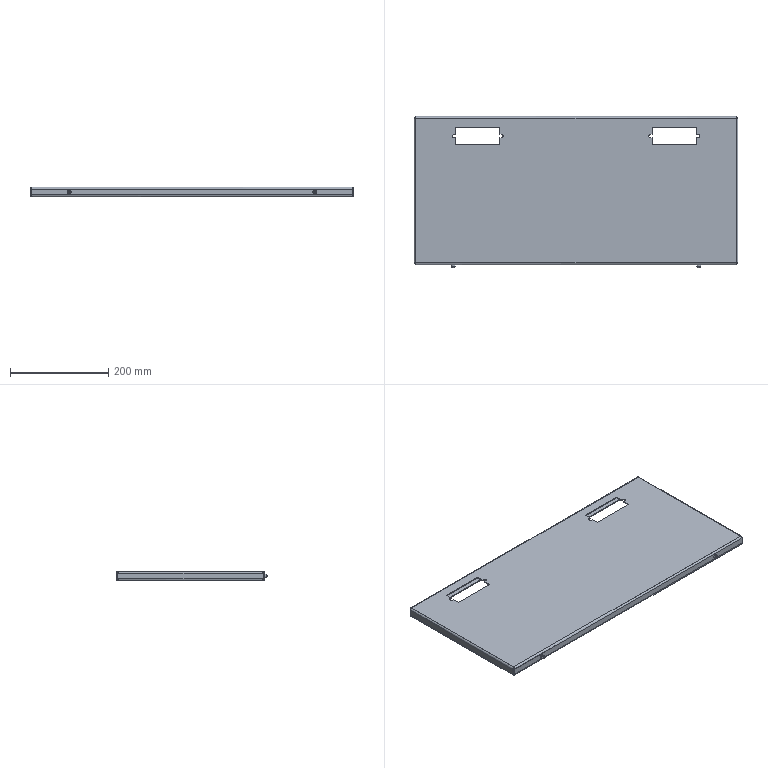Part | NX | features BREP 1 | 1 solid | 106 faces | box 660 x 308 x 20 mm | volume 492535 mm3 | plane 60 | cylinder 26 | spline 16 | cone 4 | commonest cylinder face diameters 8 x12 4 x8 7 x6